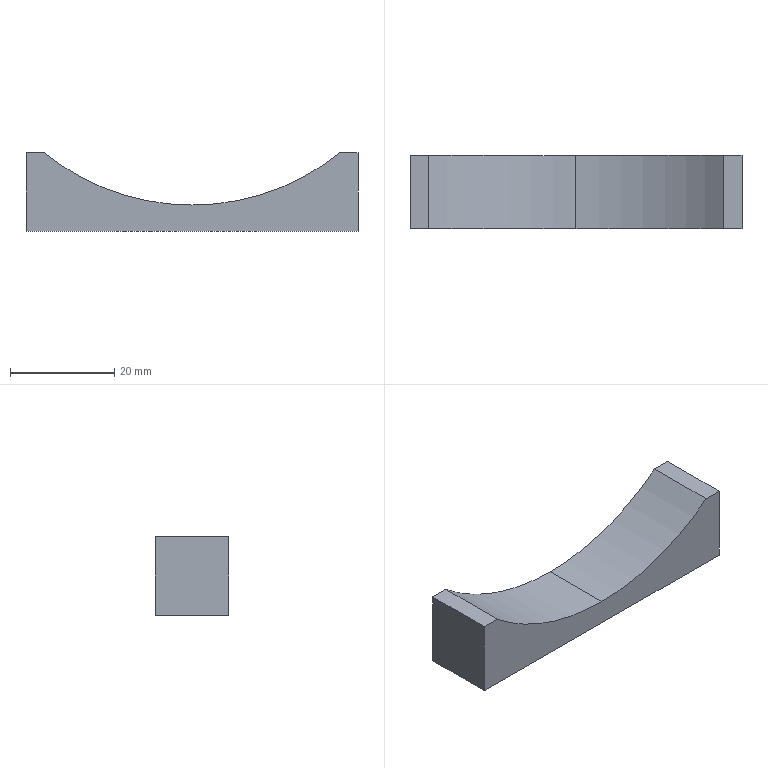Part | STEP file | Guide wheel mechanism revised.sldasm-Part-480 | 1 solid | 9 faces | box 63.64 x 14 x 15 mm | volume 7955 mm3 | plane 7 | cylinder 2 | commonest cylinder face diameters 90 x2
STEP:
#1=CARTESIAN_POINT('',(28.284,14.,-35.));
#2=VERTEX_POINT('',#1);
#3=CARTESIAN_POINT('',(0.,14.,-45.));
#4=VERTEX_POINT('',#3);
#5=CARTESIAN_POINT('',(0.,14.,0.));
#6=DIRECTION('',(0.,1.,0.));
#7=DIRECTION('',(0.,0.,1.));
#8=AXIS2_PLACEMENT_3D('',#5,#6,#7);
#9=CIRCLE('',#8,45.);
#10=EDGE_CURVE('',#2,#4,#9,.T.);
#11=ORIENTED_EDGE('',*,*,#10,.T.);
#12=CARTESIAN_POINT('',(0.,0.,-45.));
#13=VERTEX_POINT('',#12);
#14=CARTESIAN_POINT('',(0.,14.,-45.));
#15=DIRECTION('',(0.,-1.,0.));
#16=VECTOR('',#15,1000.);
#17=LINE('',#14,#16);
#18=EDGE_CURVE('',#4,#13,#17,.T.);
#19=ORIENTED_EDGE('',*,*,#18,.T.);
#20=CARTESIAN_POINT('',(28.284,0.,-35.));
#21=VERTEX_POINT('',#20);
#22=CARTESIAN_POINT('',(0.,0.,0.));
#23=DIRECTION('',(0.,1.,0.));
#24=DIRECTION('',(0.,0.,1.));
#25=AXIS2_PLACEMENT_3D('',#22,#23,#24);
#26=CIRCLE('',#25,45.);
#27=EDGE_CURVE('',#21,#13,#26,.T.);
#28=ORIENTED_EDGE('',*,*,#27,.F.);
#29=CARTESIAN_POINT('',(28.284,14.,-35.));
#30=DIRECTION('',(0.,1.,0.));
#31=VECTOR('',#30,1000.);
#32=LINE('',#29,#31);
#33=EDGE_CURVE('',#21,#2,#32,.T.);
#34=ORIENTED_EDGE('',*,*,#33,.T.);
#35=EDGE_LOOP('',(#11,#19,#28,#34));
#36=FACE_OUTER_BOUND('',#35,.T.);
#37=CARTESIAN_POINT('',(0.,14.,0.));
#38=DIRECTION('',(0.,-1.,0.));
#39=DIRECTION('',(0.,0.,-1.));
#40=AXIS2_PLACEMENT_3D('',#37,#38,#39);
#41=CYLINDRICAL_SURFACE('',#40,45.);
#42=ADVANCED_FACE('',(#36),#41,.F.);
#43=CARTESIAN_POINT('',(31.82,14.,-35.));
#44=VERTEX_POINT('',#43);
#45=CARTESIAN_POINT('',(31.82,14.,-50.));
#46=VERTEX_POINT('',#45);
#47=CARTESIAN_POINT('',(31.82,14.,-31.82));
#48=DIRECTION('',(0.,0.,-1.));
#49=VECTOR('',#48,1000.);
#50=LINE('',#47,#49);
#51=EDGE_CURVE('',#44,#46,#50,.T.);
#52=ORIENTED_EDGE('',*,*,#51,.F.);
#53=CARTESIAN_POINT('',(31.82,0.,-35.));
#54=VERTEX_POINT('',#53);
#55=CARTESIAN_POINT('',(31.82,-0.001,-35.));
#56=DIRECTION('',(0.,1.,0.));
#57=VECTOR('',#56,1000.);
#58=LINE('',#55,#57);
#59=EDGE_CURVE('',#54,#44,#58,.T.);
#60=ORIENTED_EDGE('',*,*,#59,.F.);
#61=CARTESIAN_POINT('',(31.82,0.,-50.));
#62=VERTEX_POINT('',#61);
#63=CARTESIAN_POINT('',(31.82,0.,-31.82));
#64=DIRECTION('',(0.,0.,-1.));
#65=VECTOR('',#64,1000.);
#66=LINE('',#63,#65);
#67=EDGE_CURVE('',#54,#62,#66,.T.);
#68=ORIENTED_EDGE('',*,*,#67,.T.);
#69=CARTESIAN_POINT('',(31.82,14.,-50.));
#70=DIRECTION('',(0.,-1.,0.));
#71=VECTOR('',#70,1000.);
#72=LINE('',#69,#71);
#73=EDGE_CURVE('',#46,#62,#72,.T.);
#74=ORIENTED_EDGE('',*,*,#73,.F.);
#75=EDGE_LOOP('',(#52,#60,#68,#74));
#76=FACE_OUTER_BOUND('',#75,.T.);
#77=CARTESIAN_POINT('',(31.82,14.,-31.82));
#78=DIRECTION('',(-1.,0.,0.));
#79=DIRECTION('',(0.,0.,1.));
#80=AXIS2_PLACEMENT_3D('',#77,#78,#79);
#81=PLANE('',#80);
#82=ADVANCED_FACE('',(#76),#81,.F.);
#83=CARTESIAN_POINT('',(-31.82,0.,-50.));
#84=VERTEX_POINT('',#83);
#85=CARTESIAN_POINT('',(31.82,0.,-50.));
#86=DIRECTION('',(-1.,0.,0.));
#87=VECTOR('',#86,1000.);
#88=LINE('',#85,#87);
#89=EDGE_CURVE('',#62,#84,#88,.T.);
#90=ORIENTED_EDGE('',*,*,#89,.T.);
#91=CARTESIAN_POINT('',(-31.82,14.,-50.));
#92=VERTEX_POINT('',#91);
#93=CARTESIAN_POINT('',(-31.82,14.,-50.));
#94=DIRECTION('',(0.,-1.,0.));
#95=VECTOR('',#94,1000.);
#96=LINE('',#93,#95);
#97=EDGE_CURVE('',#92,#84,#96,.T.);
#98=ORIENTED_EDGE('',*,*,#97,.F.);
#99=CARTESIAN_POINT('',(31.82,14.,-50.));
#100=DIRECTION('',(-1.,0.,0.));
#101=VECTOR('',#100,1000.);
#102=LINE('',#99,#101);
#103=EDGE_CURVE('',#46,#92,#102,.T.);
#104=ORIENTED_EDGE('',*,*,#103,.F.);
#105=ORIENTED_EDGE('',*,*,#73,.T.);
#106=EDGE_LOOP('',(#90,#98,#104,#105));
#107=FACE_OUTER_BOUND('',#106,.T.);
#108=CARTESIAN_POINT('',(31.82,14.,-50.));
#109=DIRECTION('',(0.,0.,1.));
#110=DIRECTION('',(1.,0.,0.));
#111=AXIS2_PLACEMENT_3D('',#108,#109,#110);
#112=PLANE('',#111);
#113=ADVANCED_FACE('',(#107),#112,.F.);
#114=CARTESIAN_POINT('',(-31.82,0.,-35.));
#115=VERTEX_POINT('',#114);
#116=CARTESIAN_POINT('',(-31.82,0.,-50.));
#117=DIRECTION('',(0.,0.,1.));
#118=VECTOR('',#117,1000.);
#119=LINE('',#116,#118);
#120=EDGE_CURVE('',#84,#115,#119,.T.);
#121=ORIENTED_EDGE('',*,*,#120,.T.);
#122=CARTESIAN_POINT('',(-31.82,14.,-35.));
#123=VERTEX_POINT('',#122);
#124=CARTESIAN_POINT('',(-31.82,-0.001,-35.));
#125=DIRECTION('',(0.,1.,0.));
#126=VECTOR('',#125,1000.);
#127=LINE('',#124,#126);
#128=EDGE_CURVE('',#115,#123,#127,.T.);
#129=ORIENTED_EDGE('',*,*,#128,.T.);
#130=CARTESIAN_POINT('',(-31.82,14.,-50.));
#131=DIRECTION('',(0.,0.,1.));
#132=VECTOR('',#131,1000.);
#133=LINE('',#130,#132);
#134=EDGE_CURVE('',#92,#123,#133,.T.);
#135=ORIENTED_EDGE('',*,*,#134,.F.);
#136=ORIENTED_EDGE('',*,*,#97,.T.);
#137=EDGE_LOOP('',(#121,#129,#135,#136));
#138=FACE_OUTER_BOUND('',#137,.T.);
#139=CARTESIAN_POINT('',(-31.82,14.,-50.));
#140=DIRECTION('',(1.,0.,0.));
#141=DIRECTION('',(0.,0.,-1.));
#142=AXIS2_PLACEMENT_3D('',#139,#140,#141);
#143=PLANE('',#142);
#144=ADVANCED_FACE('',(#138),#143,.F.);
#145=ORIENTED_EDGE('',*,*,#18,.F.);
#146=CARTESIAN_POINT('',(-28.284,14.,-35.));
#147=VERTEX_POINT('',#146);
#148=CARTESIAN_POINT('',(0.,14.,0.));
#149=DIRECTION('',(0.,1.,0.));
#150=DIRECTION('',(0.,0.,1.));
#151=AXIS2_PLACEMENT_3D('',#148,#149,#150);
#152=CIRCLE('',#151,45.);
#153=EDGE_CURVE('',#4,#147,#152,.T.);
#154=ORIENTED_EDGE('',*,*,#153,.T.);
#155=CARTESIAN_POINT('',(-28.284,0.,-35.));
#156=VERTEX_POINT('',#155);
#157=CARTESIAN_POINT('',(-28.284,14.,-35.));
#158=DIRECTION('',(0.,-1.,0.));
#159=VECTOR('',#158,1000.);
#160=LINE('',#157,#159);
#161=EDGE_CURVE('',#147,#156,#160,.T.);
#162=ORIENTED_EDGE('',*,*,#161,.T.);
#163=CARTESIAN_POINT('',(0.,0.,0.));
#164=DIRECTION('',(0.,1.,0.));
#165=DIRECTION('',(0.,0.,1.));
#166=AXIS2_PLACEMENT_3D('',#163,#164,#165);
#167=CIRCLE('',#166,45.);
#168=EDGE_CURVE('',#13,#156,#167,.T.);
#169=ORIENTED_EDGE('',*,*,#168,.F.);
#170=EDGE_LOOP('',(#145,#154,#162,#169));
#171=FACE_OUTER_BOUND('',#170,.T.);
#172=CARTESIAN_POINT('',(0.,14.,0.));
#173=DIRECTION('',(0.,-1.,0.));
#174=DIRECTION('',(0.,0.,-1.));
#175=AXIS2_PLACEMENT_3D('',#172,#173,#174);
#176=CYLINDRICAL_SURFACE('',#175,45.);
#177=ADVANCED_FACE('',(#171),#176,.F.);
#178=CARTESIAN_POINT('',(31.82,14.,-35.));
#179=DIRECTION('',(-1.,0.,0.));
#180=VECTOR('',#179,1000.);
#181=LINE('',#178,#180);
#182=EDGE_CURVE('',#147,#123,#181,.T.);
#183=ORIENTED_EDGE('',*,*,#182,.F.);
#184=ORIENTED_EDGE('',*,*,#153,.F.);
#185=ORIENTED_EDGE('',*,*,#10,.F.);
#186=CARTESIAN_POINT('',(31.82,14.,-35.));
#187=DIRECTION('',(-1.,0.,0.));
#188=VECTOR('',#187,1000.);
#189=LINE('',#186,#188);
#190=EDGE_CURVE('',#44,#2,#189,.T.);
#191=ORIENTED_EDGE('',*,*,#190,.F.);
#192=ORIENTED_EDGE('',*,*,#51,.T.);
#193=ORIENTED_EDGE('',*,*,#103,.T.);
#194=ORIENTED_EDGE('',*,*,#134,.T.);
#195=EDGE_LOOP('',(#183,#184,#185,#191,#192,#193,#194));
#196=FACE_OUTER_BOUND('',#195,.T.);
#197=CARTESIAN_POINT('',(0.,14.,0.));
#198=DIRECTION('',(0.,1.,0.));
#199=DIRECTION('',(0.,0.,1.));
#200=AXIS2_PLACEMENT_3D('',#197,#198,#199);
#201=PLANE('',#200);
#202=ADVANCED_FACE('',(#196),#201,.T.);
#203=ORIENTED_EDGE('',*,*,#27,.T.);
#204=ORIENTED_EDGE('',*,*,#168,.T.);
#205=CARTESIAN_POINT('',(31.82,0.,-35.));
#206=DIRECTION('',(1.,0.,0.));
#207=VECTOR('',#206,1000.);
#208=LINE('',#205,#207);
#209=EDGE_CURVE('',#115,#156,#208,.T.);
#210=ORIENTED_EDGE('',*,*,#209,.F.);
#211=ORIENTED_EDGE('',*,*,#120,.F.);
#212=ORIENTED_EDGE('',*,*,#89,.F.);
#213=ORIENTED_EDGE('',*,*,#67,.F.);
#214=CARTESIAN_POINT('',(31.82,0.,-35.));
#215=DIRECTION('',(1.,0.,0.));
#216=VECTOR('',#215,1000.);
#217=LINE('',#214,#216);
#218=EDGE_CURVE('',#21,#54,#217,.T.);
#219=ORIENTED_EDGE('',*,*,#218,.F.);
#220=EDGE_LOOP('',(#203,#204,#210,#211,#212,#213,#219));
#221=FACE_OUTER_BOUND('',#220,.T.);
#222=CARTESIAN_POINT('',(0.,0.,0.));
#223=DIRECTION('',(0.,1.,0.));
#224=DIRECTION('',(0.,0.,1.));
#225=AXIS2_PLACEMENT_3D('',#222,#223,#224);
#226=PLANE('',#225);
#227=ADVANCED_FACE('',(#221),#226,.F.);
#228=ORIENTED_EDGE('',*,*,#218,.T.);
#229=ORIENTED_EDGE('',*,*,#59,.T.);
#230=ORIENTED_EDGE('',*,*,#190,.T.);
#231=ORIENTED_EDGE('',*,*,#33,.F.);
#232=EDGE_LOOP('',(#228,#229,#230,#231));
#233=FACE_OUTER_BOUND('',#232,.T.);
#234=CARTESIAN_POINT('',(31.82,-0.001,-35.));
#235=DIRECTION('',(0.,0.,-1.));
#236=DIRECTION('',(-1.,0.,0.));
#237=AXIS2_PLACEMENT_3D('',#234,#235,#236);
#238=PLANE('',#237);
#239=ADVANCED_FACE('',(#233),#238,.F.);
#240=ORIENTED_EDGE('',*,*,#182,.T.);
#241=ORIENTED_EDGE('',*,*,#128,.F.);
#242=ORIENTED_EDGE('',*,*,#209,.T.);
#243=ORIENTED_EDGE('',*,*,#161,.F.);
#244=EDGE_LOOP('',(#240,#241,#242,#243));
#245=FACE_OUTER_BOUND('',#244,.T.);
#246=CARTESIAN_POINT('',(31.82,-0.001,-35.));
#247=DIRECTION('',(0.,0.,-1.));
#248=DIRECTION('',(-1.,0.,0.));
#249=AXIS2_PLACEMENT_3D('',#246,#247,#248);
#250=PLANE('',#249);
#251=ADVANCED_FACE('',(#245),#250,.F.);
#252=CLOSED_SHELL('',(#42,#82,#113,#144,#177,#202,#227,#239,#251));
#253=MANIFOLD_SOLID_BREP('',#252);
#254=CARTESIAN_POINT('',(0.,0.,0.));
#255=DIRECTION('',(0.,0.,1.));
#256=DIRECTION('',(1.,0.,0.));
#257=AXIS2_PLACEMENT_3D('',#254,#255,#256);
#258=(LENGTH_UNIT()NAMED_UNIT(*)SI_UNIT(.MILLI.,.METRE.));
#259=UNCERTAINTY_MEASURE_WITH_UNIT(LENGTH_MEASURE(0.00001),#258,'','');
#260=(NAMED_UNIT(*)PLANE_ANGLE_UNIT()SI_UNIT($,.RADIAN.));
#261=(NAMED_UNIT(*)SI_UNIT($,.STERADIAN.)SOLID_ANGLE_UNIT());
#262=(GEOMETRIC_REPRESENTATION_CONTEXT(3)GLOBAL_UNCERTAINTY_ASSIGNED_CONTEXT((#259))GLOBAL_UNIT_ASSIGNED_CONTEXT((#258,#260,#261))REPRESENTATION_CONTEXT('',''));
#263=ADVANCED_BREP_SHAPE_REPRESENTATION('',(#253,#257),#262);